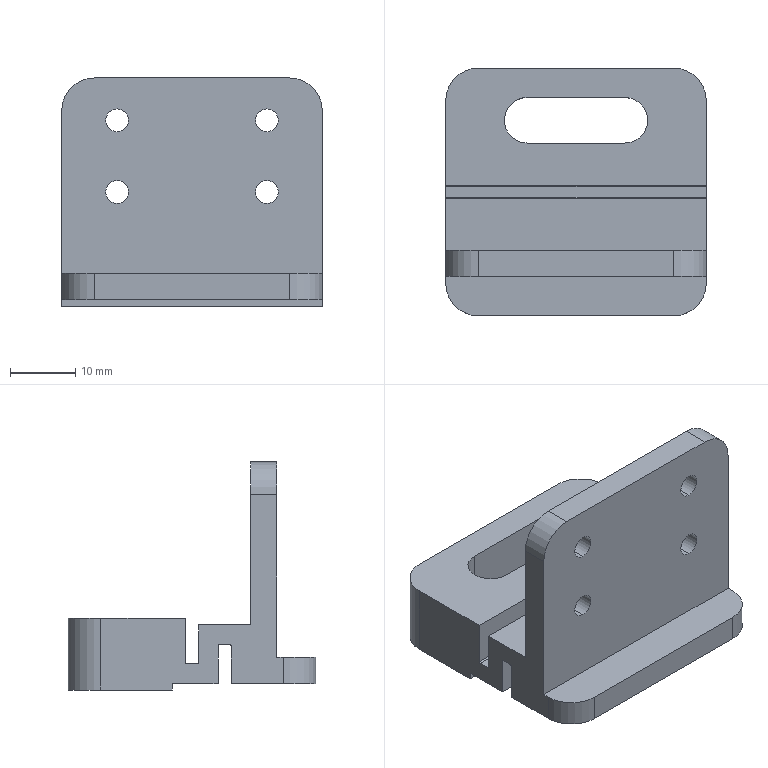Part | SolidWorks | features ICE 7, Fillet 3, MoveFace 3, Chamfer 1, Extrusion 1 | 1 solid | 51 faces | box 40 x 38 x 35 mm | volume 14882 mm3 | plane 22 | cylinder 21 | cone 8 | commonest cylinder face diameters 3.5 x8 10 x6 0.4 x4 7 x3